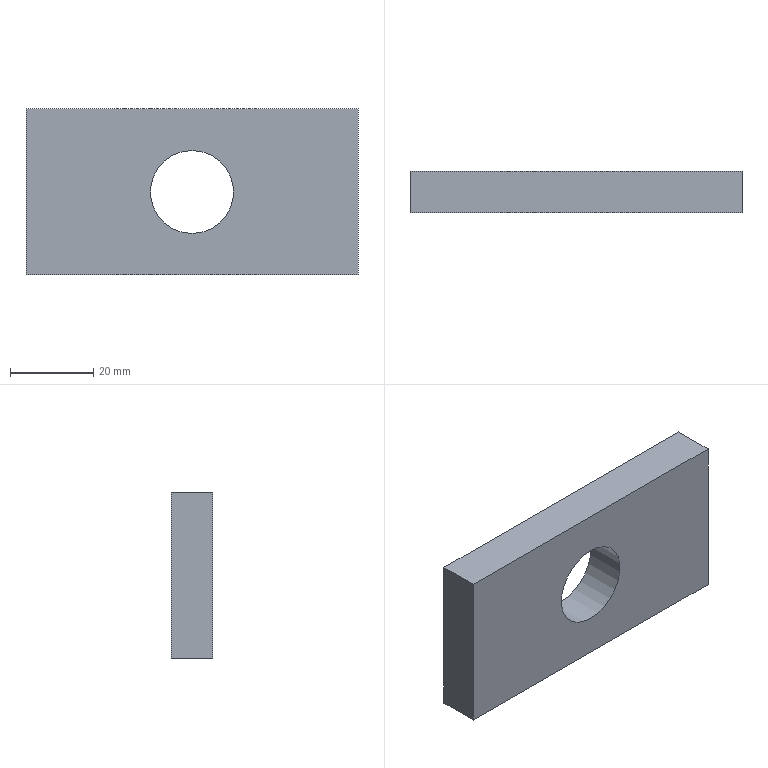Part | STEP file | dianpian | 1 solid | 7 faces | box 80 x 10 x 40 mm | volume 28858 mm3 | plane 6 | cylinder 1 | commonest cylinder face diameters 20 x1
STEP:
#1=CARTESIAN_POINT('',(0.,0.,0.));
#2=DIRECTION('',(0.,0.,1.));
#3=DIRECTION('',(1.,0.,0.));
#4=AXIS2_PLACEMENT_3D('',#1,#2,#3);
#5=CARTESIAN_POINT('',(40.,10.,20.));
#6=VERTEX_POINT('',#5);
#7=CARTESIAN_POINT('',(40.,10.,-20.));
#8=VERTEX_POINT('',#7);
#9=CARTESIAN_POINT('',(40.,10.,-20.));
#10=DIRECTION('',(0.,0.,-1.));
#11=VECTOR('',#10,1.);
#12=LINE('',#9,#11);
#13=CARTESIAN_POINT('',(0.,10.,0.));
#14=DIRECTION('',(0.,1.,0.));
#15=DIRECTION('',(0.,0.,1.));
#16=AXIS2_PLACEMENT_3D('',#13,#14,#15);
#17=PLANE('',#16);
#18=CARTESIAN_POINT('',(-20.,40.));
#19=DIRECTION('',(-1.,0.));
#20=VECTOR('',#19,1.);
#21=LINE('',#18,#20);
#22=(GEOMETRIC_REPRESENTATION_CONTEXT(2)PARAMETRIC_REPRESENTATION_CONTEXT()REPRESENTATION_CONTEXT('',''));
#23=DEFINITIONAL_REPRESENTATION('',(#21),#22);
#24=PCURVE('',#17,#23);
#25=CARTESIAN_POINT('',(40.,10.,-20.));
#26=DIRECTION('',(-1.,0.,0.));
#27=DIRECTION('',(0.,0.,1.));
#28=AXIS2_PLACEMENT_3D('',#25,#26,#27);
#29=PLANE('',#28);
#30=CARTESIAN_POINT('',(0.,0.));
#31=DIRECTION('',(-1.,0.));
#32=VECTOR('',#31,1.);
#33=LINE('',#30,#32);
#34=(GEOMETRIC_REPRESENTATION_CONTEXT(2)PARAMETRIC_REPRESENTATION_CONTEXT()REPRESENTATION_CONTEXT('',''));
#35=DEFINITIONAL_REPRESENTATION('',(#33),#34);
#36=PCURVE('',#29,#35);
#37=SURFACE_CURVE('',#12,(#24,#36),.PCURVE_S1.);
#38=EDGE_CURVE('',#6,#8,#37,.T.);
#39=ORIENTED_EDGE('',*,*,#38,.T.);
#40=CARTESIAN_POINT('',(-40.,10.,-20.));
#41=VERTEX_POINT('',#40);
#42=CARTESIAN_POINT('',(-40.,10.,-20.));
#43=DIRECTION('',(-1.,0.,0.));
#44=VECTOR('',#43,1.);
#45=LINE('',#42,#44);
#46=CARTESIAN_POINT('',(-20.,-40.));
#47=DIRECTION('',(0.,-1.));
#48=VECTOR('',#47,1.);
#49=LINE('',#46,#48);
#50=(GEOMETRIC_REPRESENTATION_CONTEXT(2)PARAMETRIC_REPRESENTATION_CONTEXT()REPRESENTATION_CONTEXT('',''));
#51=DEFINITIONAL_REPRESENTATION('',(#49),#50);
#52=PCURVE('',#17,#51);
#53=CARTESIAN_POINT('',(-40.,10.,-20.));
#54=DIRECTION('',(0.,0.,1.));
#55=DIRECTION('',(1.,0.,0.));
#56=AXIS2_PLACEMENT_3D('',#53,#54,#55);
#57=PLANE('',#56);
#58=CARTESIAN_POINT('',(0.,0.));
#59=DIRECTION('',(-1.,0.));
#60=VECTOR('',#59,1.);
#61=LINE('',#58,#60);
#62=(GEOMETRIC_REPRESENTATION_CONTEXT(2)PARAMETRIC_REPRESENTATION_CONTEXT()REPRESENTATION_CONTEXT('',''));
#63=DEFINITIONAL_REPRESENTATION('',(#61),#62);
#64=PCURVE('',#57,#63);
#65=SURFACE_CURVE('',#45,(#52,#64),.PCURVE_S1.);
#66=EDGE_CURVE('',#8,#41,#65,.T.);
#67=ORIENTED_EDGE('',*,*,#66,.T.);
#68=CARTESIAN_POINT('',(-40.,10.,20.));
#69=VERTEX_POINT('',#68);
#70=CARTESIAN_POINT('',(-40.,10.,-20.));
#71=DIRECTION('',(0.,0.,1.));
#72=VECTOR('',#71,1.);
#73=LINE('',#70,#72);
#74=CARTESIAN_POINT('',(-20.,-40.));
#75=DIRECTION('',(1.,0.));
#76=VECTOR('',#75,1.);
#77=LINE('',#74,#76);
#78=(GEOMETRIC_REPRESENTATION_CONTEXT(2)PARAMETRIC_REPRESENTATION_CONTEXT()REPRESENTATION_CONTEXT('',''));
#79=DEFINITIONAL_REPRESENTATION('',(#77),#78);
#80=PCURVE('',#17,#79);
#81=CARTESIAN_POINT('',(-40.,10.,-20.));
#82=DIRECTION('',(1.,0.,0.));
#83=DIRECTION('',(0.,0.,-1.));
#84=AXIS2_PLACEMENT_3D('',#81,#82,#83);
#85=PLANE('',#84);
#86=CARTESIAN_POINT('',(0.,0.));
#87=DIRECTION('',(-1.,0.));
#88=VECTOR('',#87,1.);
#89=LINE('',#86,#88);
#90=(GEOMETRIC_REPRESENTATION_CONTEXT(2)PARAMETRIC_REPRESENTATION_CONTEXT()REPRESENTATION_CONTEXT('',''));
#91=DEFINITIONAL_REPRESENTATION('',(#89),#90);
#92=PCURVE('',#85,#91);
#93=SURFACE_CURVE('',#73,(#80,#92),.PCURVE_S1.);
#94=EDGE_CURVE('',#41,#69,#93,.T.);
#95=ORIENTED_EDGE('',*,*,#94,.T.);
#96=CARTESIAN_POINT('',(-40.,10.,20.));
#97=DIRECTION('',(1.,0.,0.));
#98=VECTOR('',#97,1.);
#99=LINE('',#96,#98);
#100=CARTESIAN_POINT('',(20.,-40.));
#101=DIRECTION('',(0.,1.));
#102=VECTOR('',#101,1.);
#103=LINE('',#100,#102);
#104=(GEOMETRIC_REPRESENTATION_CONTEXT(2)PARAMETRIC_REPRESENTATION_CONTEXT()REPRESENTATION_CONTEXT('',''));
#105=DEFINITIONAL_REPRESENTATION('',(#103),#104);
#106=PCURVE('',#17,#105);
#107=CARTESIAN_POINT('',(-40.,10.,20.));
#108=DIRECTION('',(0.,0.,-1.));
#109=DIRECTION('',(-1.,0.,0.));
#110=AXIS2_PLACEMENT_3D('',#107,#108,#109);
#111=PLANE('',#110);
#112=CARTESIAN_POINT('',(0.,0.));
#113=DIRECTION('',(-1.,0.));
#114=VECTOR('',#113,1.);
#115=LINE('',#112,#114);
#116=(GEOMETRIC_REPRESENTATION_CONTEXT(2)PARAMETRIC_REPRESENTATION_CONTEXT()REPRESENTATION_CONTEXT('',''));
#117=DEFINITIONAL_REPRESENTATION('',(#115),#116);
#118=PCURVE('',#111,#117);
#119=SURFACE_CURVE('',#99,(#106,#118),.PCURVE_S1.);
#120=EDGE_CURVE('',#69,#6,#119,.T.);
#121=ORIENTED_EDGE('',*,*,#120,.T.);
#122=EDGE_LOOP('',(#39,#67,#95,#121));
#123=FACE_BOUND('',#122,.T.);
#124=CARTESIAN_POINT('',(0.,10.,10.));
#125=VERTEX_POINT('',#124);
#126=CARTESIAN_POINT('',(0.,10.,0.));
#127=DIRECTION('',(0.,1.,0.));
#128=DIRECTION('',(0.,0.,1.));
#129=AXIS2_PLACEMENT_3D('',#126,#127,#128);
#130=CIRCLE('',#129,10.);
#131=CARTESIAN_POINT('',(0.,0.));
#132=DIRECTION('',(1.,0.));
#133=AXIS2_PLACEMENT_2D('',#131,#132);
#134=CIRCLE('',#133,10.);
#135=(GEOMETRIC_REPRESENTATION_CONTEXT(2)PARAMETRIC_REPRESENTATION_CONTEXT()REPRESENTATION_CONTEXT('',''));
#136=DEFINITIONAL_REPRESENTATION('',(#134),#135);
#137=PCURVE('',#17,#136);
#138=CARTESIAN_POINT('',(0.,10.,0.));
#139=DIRECTION('',(0.,-1.,0.));
#140=DIRECTION('',(0.,0.,-1.));
#141=AXIS2_PLACEMENT_3D('',#138,#139,#140);
#142=CYLINDRICAL_SURFACE('',#141,10.);
#143=CARTESIAN_POINT('',(9.425,0.));
#144=DIRECTION('',(-1.,0.));
#145=VECTOR('',#144,1.);
#146=LINE('',#143,#145);
#147=(GEOMETRIC_REPRESENTATION_CONTEXT(2)PARAMETRIC_REPRESENTATION_CONTEXT()REPRESENTATION_CONTEXT('',''));
#148=DEFINITIONAL_REPRESENTATION('',(#146),#147);
#149=PCURVE('',#142,#148);
#150=SURFACE_CURVE('',#130,(#137,#149),.PCURVE_S1.);
#151=EDGE_CURVE('',#125,#125,#150,.T.);
#152=ORIENTED_EDGE('',*,*,#151,.F.);
#153=EDGE_LOOP('',(#152));
#154=FACE_BOUND('',#153,.T.);
#155=ADVANCED_FACE('',(#123,#154),#17,.T.);
#156=CARTESIAN_POINT('',(40.,0.,20.));
#157=VERTEX_POINT('',#156);
#158=CARTESIAN_POINT('',(40.,0.,-20.));
#159=VERTEX_POINT('',#158);
#160=CARTESIAN_POINT('',(40.,0.,-20.));
#161=DIRECTION('',(0.,0.,-1.));
#162=VECTOR('',#161,1.);
#163=LINE('',#160,#162);
#164=CARTESIAN_POINT('',(0.,0.,0.));
#165=DIRECTION('',(0.,1.,0.));
#166=DIRECTION('',(0.,0.,1.));
#167=AXIS2_PLACEMENT_3D('',#164,#165,#166);
#168=PLANE('',#167);
#169=CARTESIAN_POINT('',(-20.,40.));
#170=DIRECTION('',(-1.,0.));
#171=VECTOR('',#170,1.);
#172=LINE('',#169,#171);
#173=(GEOMETRIC_REPRESENTATION_CONTEXT(2)PARAMETRIC_REPRESENTATION_CONTEXT()REPRESENTATION_CONTEXT('',''));
#174=DEFINITIONAL_REPRESENTATION('',(#172),#173);
#175=PCURVE('',#168,#174);
#176=CARTESIAN_POINT('',(0.,-10.));
#177=DIRECTION('',(-1.,0.));
#178=VECTOR('',#177,1.);
#179=LINE('',#176,#178);
#180=(GEOMETRIC_REPRESENTATION_CONTEXT(2)PARAMETRIC_REPRESENTATION_CONTEXT()REPRESENTATION_CONTEXT('',''));
#181=DEFINITIONAL_REPRESENTATION('',(#179),#180);
#182=PCURVE('',#29,#181);
#183=SURFACE_CURVE('',#163,(#175,#182),.PCURVE_S1.);
#184=EDGE_CURVE('',#157,#159,#183,.T.);
#185=ORIENTED_EDGE('',*,*,#184,.F.);
#186=CARTESIAN_POINT('',(-40.,0.,20.));
#187=VERTEX_POINT('',#186);
#188=CARTESIAN_POINT('',(-40.,0.,20.));
#189=DIRECTION('',(1.,0.,0.));
#190=VECTOR('',#189,1.);
#191=LINE('',#188,#190);
#192=CARTESIAN_POINT('',(20.,-40.));
#193=DIRECTION('',(0.,1.));
#194=VECTOR('',#193,1.);
#195=LINE('',#192,#194);
#196=(GEOMETRIC_REPRESENTATION_CONTEXT(2)PARAMETRIC_REPRESENTATION_CONTEXT()REPRESENTATION_CONTEXT('',''));
#197=DEFINITIONAL_REPRESENTATION('',(#195),#196);
#198=PCURVE('',#168,#197);
#199=CARTESIAN_POINT('',(0.,-10.));
#200=DIRECTION('',(-1.,0.));
#201=VECTOR('',#200,1.);
#202=LINE('',#199,#201);
#203=(GEOMETRIC_REPRESENTATION_CONTEXT(2)PARAMETRIC_REPRESENTATION_CONTEXT()REPRESENTATION_CONTEXT('',''));
#204=DEFINITIONAL_REPRESENTATION('',(#202),#203);
#205=PCURVE('',#111,#204);
#206=SURFACE_CURVE('',#191,(#198,#205),.PCURVE_S1.);
#207=EDGE_CURVE('',#187,#157,#206,.T.);
#208=ORIENTED_EDGE('',*,*,#207,.F.);
#209=CARTESIAN_POINT('',(-40.,0.,-20.));
#210=VERTEX_POINT('',#209);
#211=CARTESIAN_POINT('',(-40.,0.,-20.));
#212=DIRECTION('',(0.,0.,1.));
#213=VECTOR('',#212,1.);
#214=LINE('',#211,#213);
#215=CARTESIAN_POINT('',(-20.,-40.));
#216=DIRECTION('',(1.,0.));
#217=VECTOR('',#216,1.);
#218=LINE('',#215,#217);
#219=(GEOMETRIC_REPRESENTATION_CONTEXT(2)PARAMETRIC_REPRESENTATION_CONTEXT()REPRESENTATION_CONTEXT('',''));
#220=DEFINITIONAL_REPRESENTATION('',(#218),#219);
#221=PCURVE('',#168,#220);
#222=CARTESIAN_POINT('',(0.,-10.));
#223=DIRECTION('',(-1.,0.));
#224=VECTOR('',#223,1.);
#225=LINE('',#222,#224);
#226=(GEOMETRIC_REPRESENTATION_CONTEXT(2)PARAMETRIC_REPRESENTATION_CONTEXT()REPRESENTATION_CONTEXT('',''));
#227=DEFINITIONAL_REPRESENTATION('',(#225),#226);
#228=PCURVE('',#85,#227);
#229=SURFACE_CURVE('',#214,(#221,#228),.PCURVE_S1.);
#230=EDGE_CURVE('',#210,#187,#229,.T.);
#231=ORIENTED_EDGE('',*,*,#230,.F.);
#232=CARTESIAN_POINT('',(-40.,0.,-20.));
#233=DIRECTION('',(-1.,0.,0.));
#234=VECTOR('',#233,1.);
#235=LINE('',#232,#234);
#236=CARTESIAN_POINT('',(-20.,-40.));
#237=DIRECTION('',(0.,-1.));
#238=VECTOR('',#237,1.);
#239=LINE('',#236,#238);
#240=(GEOMETRIC_REPRESENTATION_CONTEXT(2)PARAMETRIC_REPRESENTATION_CONTEXT()REPRESENTATION_CONTEXT('',''));
#241=DEFINITIONAL_REPRESENTATION('',(#239),#240);
#242=PCURVE('',#168,#241);
#243=CARTESIAN_POINT('',(0.,-10.));
#244=DIRECTION('',(-1.,0.));
#245=VECTOR('',#244,1.);
#246=LINE('',#243,#245);
#247=(GEOMETRIC_REPRESENTATION_CONTEXT(2)PARAMETRIC_REPRESENTATION_CONTEXT()REPRESENTATION_CONTEXT('',''));
#248=DEFINITIONAL_REPRESENTATION('',(#246),#247);
#249=PCURVE('',#57,#248);
#250=SURFACE_CURVE('',#235,(#242,#249),.PCURVE_S1.);
#251=EDGE_CURVE('',#159,#210,#250,.T.);
#252=ORIENTED_EDGE('',*,*,#251,.F.);
#253=EDGE_LOOP('',(#185,#208,#231,#252));
#254=FACE_BOUND('',#253,.T.);
#255=CARTESIAN_POINT('',(0.,0.,10.));
#256=VERTEX_POINT('',#255);
#257=CARTESIAN_POINT('',(0.,0.,0.));
#258=DIRECTION('',(0.,1.,0.));
#259=DIRECTION('',(0.,0.,1.));
#260=AXIS2_PLACEMENT_3D('',#257,#258,#259);
#261=CIRCLE('',#260,10.);
#262=CARTESIAN_POINT('',(0.,0.));
#263=DIRECTION('',(1.,0.));
#264=AXIS2_PLACEMENT_2D('',#262,#263);
#265=CIRCLE('',#264,10.);
#266=(GEOMETRIC_REPRESENTATION_CONTEXT(2)PARAMETRIC_REPRESENTATION_CONTEXT()REPRESENTATION_CONTEXT('',''));
#267=DEFINITIONAL_REPRESENTATION('',(#265),#266);
#268=PCURVE('',#168,#267);
#269=CARTESIAN_POINT('',(9.425,10.));
#270=DIRECTION('',(-1.,0.));
#271=VECTOR('',#270,1.);
#272=LINE('',#269,#271);
#273=(GEOMETRIC_REPRESENTATION_CONTEXT(2)PARAMETRIC_REPRESENTATION_CONTEXT()REPRESENTATION_CONTEXT('',''));
#274=DEFINITIONAL_REPRESENTATION('',(#272),#273);
#275=PCURVE('',#142,#274);
#276=SURFACE_CURVE('',#261,(#268,#275),.PCURVE_S1.);
#277=EDGE_CURVE('',#256,#256,#276,.T.);
#278=ORIENTED_EDGE('',*,*,#277,.T.);
#279=EDGE_LOOP('',(#278));
#280=FACE_BOUND('',#279,.T.);
#281=ADVANCED_FACE('',(#254,#280),#168,.F.);
#282=ORIENTED_EDGE('',*,*,#184,.T.);
#283=CARTESIAN_POINT('',(40.,10.,-20.));
#284=DIRECTION('',(0.,-1.,0.));
#285=VECTOR('',#284,1.);
#286=LINE('',#283,#285);
#287=CARTESIAN_POINT('',(0.,0.));
#288=DIRECTION('',(0.,-1.));
#289=VECTOR('',#288,1.);
#290=LINE('',#287,#289);
#291=(GEOMETRIC_REPRESENTATION_CONTEXT(2)PARAMETRIC_REPRESENTATION_CONTEXT()REPRESENTATION_CONTEXT('',''));
#292=DEFINITIONAL_REPRESENTATION('',(#290),#291);
#293=PCURVE('',#29,#292);
#294=CARTESIAN_POINT('',(80.,0.));
#295=DIRECTION('',(0.,-1.));
#296=VECTOR('',#295,1.);
#297=LINE('',#294,#296);
#298=(GEOMETRIC_REPRESENTATION_CONTEXT(2)PARAMETRIC_REPRESENTATION_CONTEXT()REPRESENTATION_CONTEXT('',''));
#299=DEFINITIONAL_REPRESENTATION('',(#297),#298);
#300=PCURVE('',#57,#299);
#301=SURFACE_CURVE('',#286,(#293,#300),.PCURVE_S1.);
#302=EDGE_CURVE('',#8,#159,#301,.T.);
#303=ORIENTED_EDGE('',*,*,#302,.F.);
#304=ORIENTED_EDGE('',*,*,#38,.F.);
#305=CARTESIAN_POINT('',(40.,10.,20.));
#306=DIRECTION('',(0.,-1.,0.));
#307=VECTOR('',#306,1.);
#308=LINE('',#305,#307);
#309=CARTESIAN_POINT('',(40.,0.));
#310=DIRECTION('',(0.,-1.));
#311=VECTOR('',#310,1.);
#312=LINE('',#309,#311);
#313=(GEOMETRIC_REPRESENTATION_CONTEXT(2)PARAMETRIC_REPRESENTATION_CONTEXT()REPRESENTATION_CONTEXT('',''));
#314=DEFINITIONAL_REPRESENTATION('',(#312),#313);
#315=PCURVE('',#29,#314);
#316=CARTESIAN_POINT('',(-80.,0.));
#317=DIRECTION('',(0.,-1.));
#318=VECTOR('',#317,1.);
#319=LINE('',#316,#318);
#320=(GEOMETRIC_REPRESENTATION_CONTEXT(2)PARAMETRIC_REPRESENTATION_CONTEXT()REPRESENTATION_CONTEXT('',''));
#321=DEFINITIONAL_REPRESENTATION('',(#319),#320);
#322=PCURVE('',#111,#321);
#323=SURFACE_CURVE('',#308,(#315,#322),.PCURVE_S1.);
#324=EDGE_CURVE('',#6,#157,#323,.T.);
#325=ORIENTED_EDGE('',*,*,#324,.T.);
#326=EDGE_LOOP('',(#282,#303,#304,#325));
#327=FACE_BOUND('',#326,.T.);
#328=ADVANCED_FACE('',(#327),#29,.F.);
#329=ORIENTED_EDGE('',*,*,#251,.T.);
#330=CARTESIAN_POINT('',(-40.,10.,-20.));
#331=DIRECTION('',(0.,-1.,0.));
#332=VECTOR('',#331,1.);
#333=LINE('',#330,#332);
#334=CARTESIAN_POINT('',(0.,0.));
#335=DIRECTION('',(0.,-1.));
#336=VECTOR('',#335,1.);
#337=LINE('',#334,#336);
#338=(GEOMETRIC_REPRESENTATION_CONTEXT(2)PARAMETRIC_REPRESENTATION_CONTEXT()REPRESENTATION_CONTEXT('',''));
#339=DEFINITIONAL_REPRESENTATION('',(#337),#338);
#340=PCURVE('',#57,#339);
#341=CARTESIAN_POINT('',(0.,0.));
#342=DIRECTION('',(0.,-1.));
#343=VECTOR('',#342,1.);
#344=LINE('',#341,#343);
#345=(GEOMETRIC_REPRESENTATION_CONTEXT(2)PARAMETRIC_REPRESENTATION_CONTEXT()REPRESENTATION_CONTEXT('',''));
#346=DEFINITIONAL_REPRESENTATION('',(#344),#345);
#347=PCURVE('',#85,#346);
#348=SURFACE_CURVE('',#333,(#340,#347),.PCURVE_S1.);
#349=EDGE_CURVE('',#41,#210,#348,.T.);
#350=ORIENTED_EDGE('',*,*,#349,.F.);
#351=ORIENTED_EDGE('',*,*,#66,.F.);
#352=ORIENTED_EDGE('',*,*,#302,.T.);
#353=EDGE_LOOP('',(#329,#350,#351,#352));
#354=FACE_BOUND('',#353,.T.);
#355=ADVANCED_FACE('',(#354),#57,.F.);
#356=ORIENTED_EDGE('',*,*,#230,.T.);
#357=CARTESIAN_POINT('',(-40.,10.,20.));
#358=DIRECTION('',(0.,-1.,0.));
#359=VECTOR('',#358,1.);
#360=LINE('',#357,#359);
#361=CARTESIAN_POINT('',(-40.,0.));
#362=DIRECTION('',(0.,-1.));
#363=VECTOR('',#362,1.);
#364=LINE('',#361,#363);
#365=(GEOMETRIC_REPRESENTATION_CONTEXT(2)PARAMETRIC_REPRESENTATION_CONTEXT()REPRESENTATION_CONTEXT('',''));
#366=DEFINITIONAL_REPRESENTATION('',(#364),#365);
#367=PCURVE('',#85,#366);
#368=CARTESIAN_POINT('',(0.,0.));
#369=DIRECTION('',(0.,-1.));
#370=VECTOR('',#369,1.);
#371=LINE('',#368,#370);
#372=(GEOMETRIC_REPRESENTATION_CONTEXT(2)PARAMETRIC_REPRESENTATION_CONTEXT()REPRESENTATION_CONTEXT('',''));
#373=DEFINITIONAL_REPRESENTATION('',(#371),#372);
#374=PCURVE('',#111,#373);
#375=SURFACE_CURVE('',#360,(#367,#374),.PCURVE_S1.);
#376=EDGE_CURVE('',#69,#187,#375,.T.);
#377=ORIENTED_EDGE('',*,*,#376,.F.);
#378=ORIENTED_EDGE('',*,*,#94,.F.);
#379=ORIENTED_EDGE('',*,*,#349,.T.);
#380=EDGE_LOOP('',(#356,#377,#378,#379));
#381=FACE_BOUND('',#380,.T.);
#382=ADVANCED_FACE('',(#381),#85,.F.);
#383=ORIENTED_EDGE('',*,*,#207,.T.);
#384=ORIENTED_EDGE('',*,*,#324,.F.);
#385=ORIENTED_EDGE('',*,*,#120,.F.);
#386=ORIENTED_EDGE('',*,*,#376,.T.);
#387=EDGE_LOOP('',(#383,#384,#385,#386));
#388=FACE_BOUND('',#387,.T.);
#389=ADVANCED_FACE('',(#388),#111,.F.);
#390=ORIENTED_EDGE('',*,*,#151,.F.);
#391=CARTESIAN_POINT('',(0.,10.,10.));
#392=CARTESIAN_POINT('',(0.,0.,10.));
#393=B_SPLINE_CURVE_WITH_KNOTS('',1,(#391,#392),.UNSPECIFIED.,.F.,.F.,(2,2),(0.,10.),.PIECEWISE_BEZIER_KNOTS.);
#394=CARTESIAN_POINT('',(9.425,0.));
#395=DIRECTION('',(0.,1.));
#396=VECTOR('',#395,1.);
#397=LINE('',#394,#396);
#398=(GEOMETRIC_REPRESENTATION_CONTEXT(2)PARAMETRIC_REPRESENTATION_CONTEXT()REPRESENTATION_CONTEXT('',''));
#399=DEFINITIONAL_REPRESENTATION('',(#397),#398);
#400=PCURVE('',#142,#399);
#401=CARTESIAN_POINT('',(3.142,0.));
#402=DIRECTION('',(0.,1.));
#403=VECTOR('',#402,1.);
#404=LINE('',#401,#403);
#405=(GEOMETRIC_REPRESENTATION_CONTEXT(2)PARAMETRIC_REPRESENTATION_CONTEXT()REPRESENTATION_CONTEXT('',''));
#406=DEFINITIONAL_REPRESENTATION('',(#404),#405);
#407=PCURVE('',#142,#406);
#408=SEAM_CURVE('',#393,(#400,#407),.PCURVE_S1.);
#409=EDGE_CURVE('',#125,#256,#408,.T.);
#410=ORIENTED_EDGE('',*,*,#409,.T.);
#411=ORIENTED_EDGE('',*,*,#277,.T.);
#412=ORIENTED_EDGE('',*,*,#409,.F.);
#413=EDGE_LOOP('',(#390,#410,#411,#412));
#414=FACE_BOUND('',#413,.F.);
#415=ADVANCED_FACE('',(#414),#142,.F.);
#416=CLOSED_SHELL('',(#155,#281,#328,#355,#382,#389,#415));
#417=MANIFOLD_SOLID_BREP('',#416);
#418=(LENGTH_UNIT()NAMED_UNIT(*)SI_UNIT(.MILLI.,.METRE.));
#419=UNCERTAINTY_MEASURE_WITH_UNIT(LENGTH_MEASURE(0.000002),#418,'','');
#420=(NAMED_UNIT(*)PLANE_ANGLE_UNIT()SI_UNIT($,.RADIAN.));
#421=(NAMED_UNIT(*)SI_UNIT($,.STERADIAN.)SOLID_ANGLE_UNIT());
#422=(GEOMETRIC_REPRESENTATION_CONTEXT(3)GLOBAL_UNCERTAINTY_ASSIGNED_CONTEXT((#419))GLOBAL_UNIT_ASSIGNED_CONTEXT((#418,#420,#421))REPRESENTATION_CONTEXT('',''));
#423=ADVANCED_BREP_SHAPE_REPRESENTATION('',(#4,#417),#422);